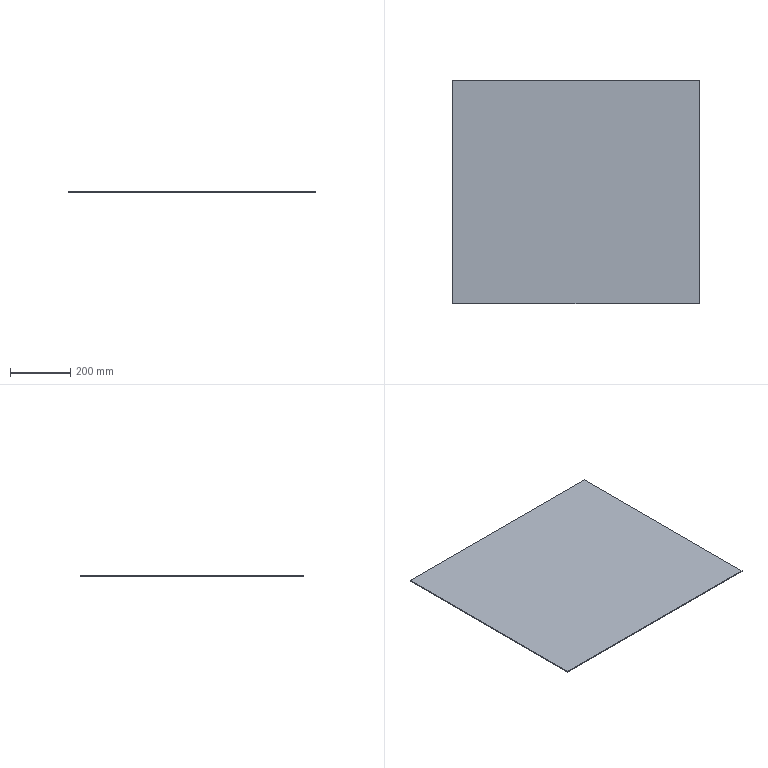Part | SolidWorks | features Extrusion 1 | 1 solid | 6 faces | box 817.222 x 740.222 x 3 mm | volume 1814778 mm3 | plane 6
STEP:
#1=CARTESIAN_POINT('',(408.611,-370.111,0.));
#2=VERTEX_POINT('',#1);
#3=CARTESIAN_POINT('',(408.611,370.111,0.));
#4=VERTEX_POINT('',#3);
#5=CARTESIAN_POINT('',(408.611,370.111,0.));
#6=DIRECTION('',(0.,1.,0.));
#7=VECTOR('',#6,1000.);
#8=LINE('',#5,#7);
#9=EDGE_CURVE('',#2,#4,#8,.T.);
#10=ORIENTED_EDGE('',*,*,#9,.T.);
#11=CARTESIAN_POINT('',(408.611,370.111,3.));
#12=VERTEX_POINT('',#11);
#13=CARTESIAN_POINT('',(408.611,370.111,3.));
#14=DIRECTION('',(0.,0.,-1.));
#15=VECTOR('',#14,1000.);
#16=LINE('',#13,#15);
#17=EDGE_CURVE('',#12,#4,#16,.T.);
#18=ORIENTED_EDGE('',*,*,#17,.F.);
#19=CARTESIAN_POINT('',(408.611,-370.111,3.));
#20=VERTEX_POINT('',#19);
#21=CARTESIAN_POINT('',(408.611,370.111,3.));
#22=DIRECTION('',(0.,1.,0.));
#23=VECTOR('',#22,1000.);
#24=LINE('',#21,#23);
#25=EDGE_CURVE('',#20,#12,#24,.T.);
#26=ORIENTED_EDGE('',*,*,#25,.F.);
#27=CARTESIAN_POINT('',(408.611,-370.111,3.));
#28=DIRECTION('',(0.,0.,-1.));
#29=VECTOR('',#28,1000.);
#30=LINE('',#27,#29);
#31=EDGE_CURVE('',#20,#2,#30,.T.);
#32=ORIENTED_EDGE('',*,*,#31,.T.);
#33=EDGE_LOOP('',(#10,#18,#26,#32));
#34=FACE_OUTER_BOUND('',#33,.T.);
#35=CARTESIAN_POINT('',(408.611,370.111,3.));
#36=DIRECTION('',(-1.,0.,0.));
#37=DIRECTION('',(0.,-1.,0.));
#38=AXIS2_PLACEMENT_3D('',#35,#36,#37);
#39=PLANE('',#38);
#40=ADVANCED_FACE('',(#34),#39,.F.);
#41=CARTESIAN_POINT('',(-408.611,370.111,0.));
#42=VERTEX_POINT('',#41);
#43=CARTESIAN_POINT('',(-408.611,370.111,0.));
#44=DIRECTION('',(-1.,0.,0.));
#45=VECTOR('',#44,1000.);
#46=LINE('',#43,#45);
#47=EDGE_CURVE('',#4,#42,#46,.T.);
#48=ORIENTED_EDGE('',*,*,#47,.T.);
#49=CARTESIAN_POINT('',(-408.611,370.111,3.));
#50=VERTEX_POINT('',#49);
#51=CARTESIAN_POINT('',(-408.611,370.111,3.));
#52=DIRECTION('',(0.,0.,-1.));
#53=VECTOR('',#52,1000.);
#54=LINE('',#51,#53);
#55=EDGE_CURVE('',#50,#42,#54,.T.);
#56=ORIENTED_EDGE('',*,*,#55,.F.);
#57=CARTESIAN_POINT('',(-408.611,370.111,3.));
#58=DIRECTION('',(-1.,0.,0.));
#59=VECTOR('',#58,1000.);
#60=LINE('',#57,#59);
#61=EDGE_CURVE('',#12,#50,#60,.T.);
#62=ORIENTED_EDGE('',*,*,#61,.F.);
#63=ORIENTED_EDGE('',*,*,#17,.T.);
#64=EDGE_LOOP('',(#48,#56,#62,#63));
#65=FACE_OUTER_BOUND('',#64,.T.);
#66=CARTESIAN_POINT('',(-408.611,370.111,3.));
#67=DIRECTION('',(0.,-1.,0.));
#68=DIRECTION('',(0.,0.,-1.));
#69=AXIS2_PLACEMENT_3D('',#66,#67,#68);
#70=PLANE('',#69);
#71=ADVANCED_FACE('',(#65),#70,.F.);
#72=CARTESIAN_POINT('',(-408.611,-370.111,0.));
#73=VERTEX_POINT('',#72);
#74=CARTESIAN_POINT('',(-408.611,370.111,0.));
#75=DIRECTION('',(0.,-1.,0.));
#76=VECTOR('',#75,1000.);
#77=LINE('',#74,#76);
#78=EDGE_CURVE('',#42,#73,#77,.T.);
#79=ORIENTED_EDGE('',*,*,#78,.T.);
#80=CARTESIAN_POINT('',(-408.611,-370.111,3.));
#81=VERTEX_POINT('',#80);
#82=CARTESIAN_POINT('',(-408.611,-370.111,3.));
#83=DIRECTION('',(0.,0.,-1.));
#84=VECTOR('',#83,1000.);
#85=LINE('',#82,#84);
#86=EDGE_CURVE('',#81,#73,#85,.T.);
#87=ORIENTED_EDGE('',*,*,#86,.F.);
#88=CARTESIAN_POINT('',(-408.611,370.111,3.));
#89=DIRECTION('',(0.,-1.,0.));
#90=VECTOR('',#89,1000.);
#91=LINE('',#88,#90);
#92=EDGE_CURVE('',#50,#81,#91,.T.);
#93=ORIENTED_EDGE('',*,*,#92,.F.);
#94=ORIENTED_EDGE('',*,*,#55,.T.);
#95=EDGE_LOOP('',(#79,#87,#93,#94));
#96=FACE_OUTER_BOUND('',#95,.T.);
#97=CARTESIAN_POINT('',(-408.611,370.111,3.));
#98=DIRECTION('',(1.,0.,0.));
#99=DIRECTION('',(0.,1.,0.));
#100=AXIS2_PLACEMENT_3D('',#97,#98,#99);
#101=PLANE('',#100);
#102=ADVANCED_FACE('',(#96),#101,.F.);
#103=CARTESIAN_POINT('',(-408.611,-370.111,0.));
#104=DIRECTION('',(1.,0.,0.));
#105=VECTOR('',#104,1000.);
#106=LINE('',#103,#105);
#107=EDGE_CURVE('',#73,#2,#106,.T.);
#108=ORIENTED_EDGE('',*,*,#107,.T.);
#109=ORIENTED_EDGE('',*,*,#31,.F.);
#110=CARTESIAN_POINT('',(-408.611,-370.111,3.));
#111=DIRECTION('',(1.,0.,0.));
#112=VECTOR('',#111,1000.);
#113=LINE('',#110,#112);
#114=EDGE_CURVE('',#81,#20,#113,.T.);
#115=ORIENTED_EDGE('',*,*,#114,.F.);
#116=ORIENTED_EDGE('',*,*,#86,.T.);
#117=EDGE_LOOP('',(#108,#109,#115,#116));
#118=FACE_OUTER_BOUND('',#117,.T.);
#119=CARTESIAN_POINT('',(-408.611,-370.111,3.));
#120=DIRECTION('',(0.,1.,0.));
#121=DIRECTION('',(0.,0.,1.));
#122=AXIS2_PLACEMENT_3D('',#119,#120,#121);
#123=PLANE('',#122);
#124=ADVANCED_FACE('',(#118),#123,.F.);
#125=ORIENTED_EDGE('',*,*,#25,.T.);
#126=ORIENTED_EDGE('',*,*,#61,.T.);
#127=ORIENTED_EDGE('',*,*,#92,.T.);
#128=ORIENTED_EDGE('',*,*,#114,.T.);
#129=EDGE_LOOP('',(#125,#126,#127,#128));
#130=FACE_OUTER_BOUND('',#129,.T.);
#131=CARTESIAN_POINT('',(0.,0.,3.));
#132=DIRECTION('',(0.,0.,1.));
#133=DIRECTION('',(1.,0.,0.));
#134=AXIS2_PLACEMENT_3D('',#131,#132,#133);
#135=PLANE('',#134);
#136=ADVANCED_FACE('',(#130),#135,.T.);
#137=ORIENTED_EDGE('',*,*,#9,.F.);
#138=ORIENTED_EDGE('',*,*,#107,.F.);
#139=ORIENTED_EDGE('',*,*,#78,.F.);
#140=ORIENTED_EDGE('',*,*,#47,.F.);
#141=EDGE_LOOP('',(#137,#138,#139,#140));
#142=FACE_OUTER_BOUND('',#141,.T.);
#143=CARTESIAN_POINT('',(0.,0.,0.));
#144=DIRECTION('',(0.,0.,1.));
#145=DIRECTION('',(1.,0.,0.));
#146=AXIS2_PLACEMENT_3D('',#143,#144,#145);
#147=PLANE('',#146);
#148=ADVANCED_FACE('',(#142),#147,.F.);
#149=CLOSED_SHELL('',(#40,#71,#102,#124,#136,#148));
#150=MANIFOLD_SOLID_BREP('',#149);
#151=CARTESIAN_POINT('',(0.,0.,0.));
#152=DIRECTION('',(0.,0.,1.));
#153=DIRECTION('',(1.,0.,0.));
#154=AXIS2_PLACEMENT_3D('',#151,#152,#153);
#155=(LENGTH_UNIT()NAMED_UNIT(*)SI_UNIT(.MILLI.,.METRE.));
#156=UNCERTAINTY_MEASURE_WITH_UNIT(LENGTH_MEASURE(0.00001),#155,'','');
#157=(NAMED_UNIT(*)PLANE_ANGLE_UNIT()SI_UNIT($,.RADIAN.));
#158=(NAMED_UNIT(*)SI_UNIT($,.STERADIAN.)SOLID_ANGLE_UNIT());
#159=(GEOMETRIC_REPRESENTATION_CONTEXT(3)GLOBAL_UNCERTAINTY_ASSIGNED_CONTEXT((#156))GLOBAL_UNIT_ASSIGNED_CONTEXT((#155,#157,#158))REPRESENTATION_CONTEXT('',''));
#160=ADVANCED_BREP_SHAPE_REPRESENTATION('',(#150,#154),#159);